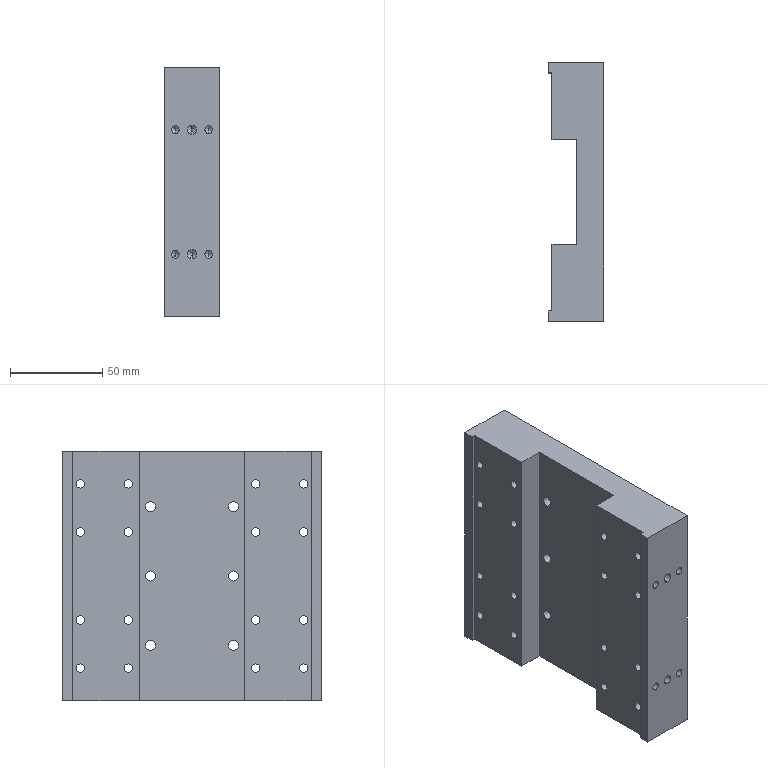Part | SolidWorks | features HoleWzd 8, ICE 2, Extrusion 1, LPattern 1 | 1 solid | 196 faces | box 30 x 140 x 135 mm | volume 401755 mm3 | cylinder 124 | cone 36 | plane 36 | commonest cylinder face diameters 4.5 x32 8 x32 4.2 x24 5.5 x12 10 x12 3.3 x8